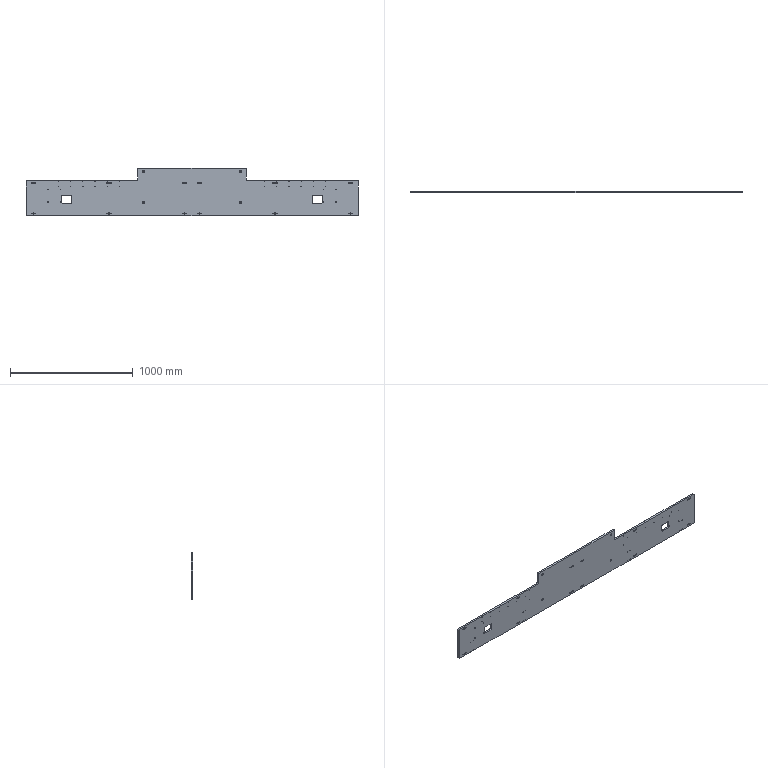Part | SolidWorks | features HoleWzd 7, ICE 4, Chamfer 1, Extrusion 1, Fillet 1, PLine 1 | 1 solid | 337 faces | box 2700 x 15 x 390 mm | volume 12856560 mm3 | cylinder 242 | cone 48 | plane 47 | commonest cylinder face diameters 3.3 x64 6.8 x64 4.2 x32 9 x24 15 x24 10 x8